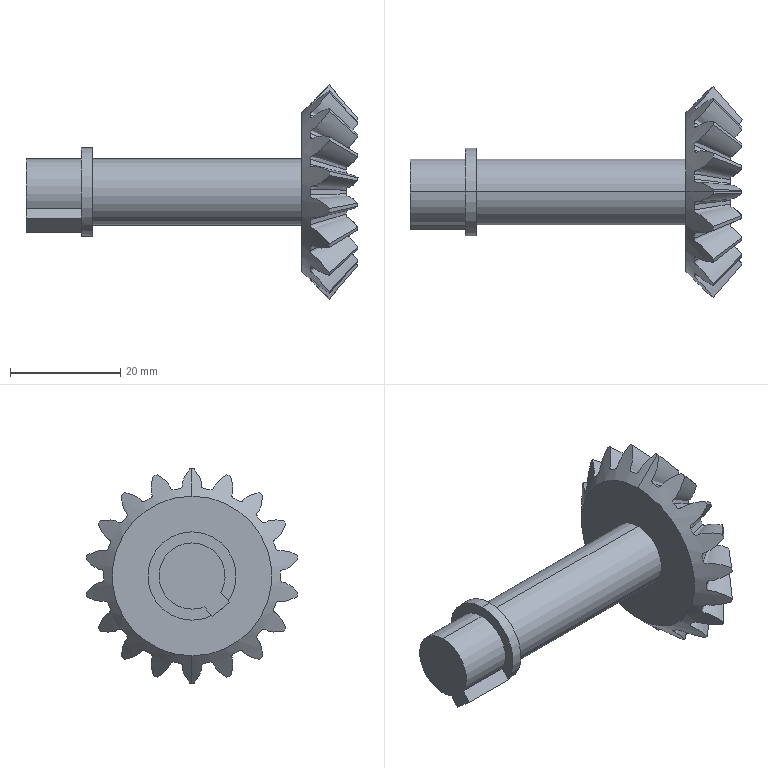Part | SolidWorks | features 3DProfileFeature 12, ICE 2, BlendCut 1, CirPattern 1, RefAxis 1, Revolution 1 | 1 solid | 114 faces | box 60.158 x 38.37 x 38.828 mm | volume 11848 mm3 | cone 40 | spline 36 | plane 29 | cylinder 9 | commonest cylinder face diameters 12 x5 7.382 x2 16 x2